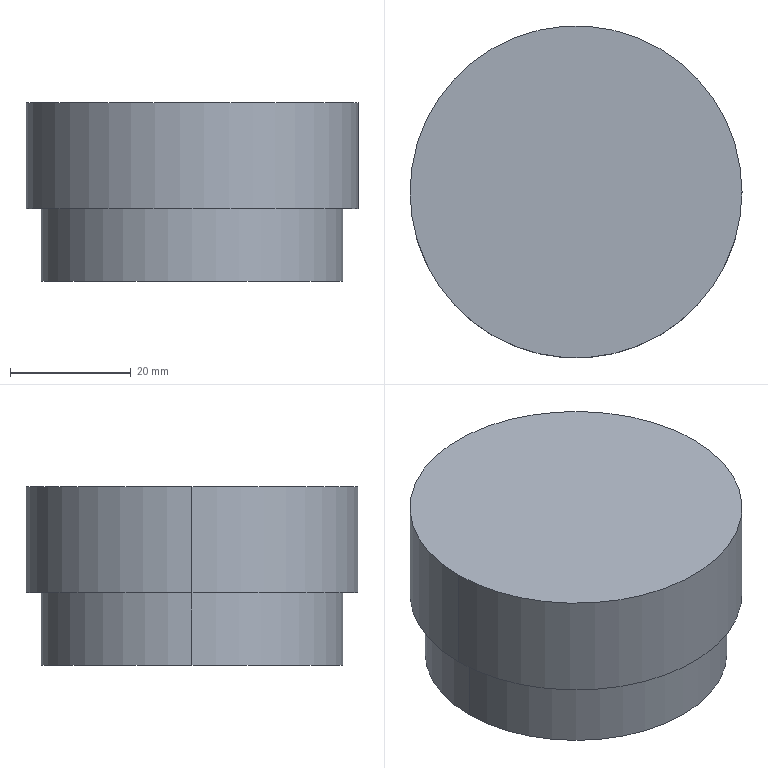Part | SolidWorks | features Extrusion 1, ICE 1 | 1 solid | 7 faces | box 55 x 55 x 29.6 mm | volume 65377 mm3 | cylinder 4 | plane 3 | commonest cylinder face diameters 50 x2 55 x2
STEP:
#1=CARTESIAN_POINT('',(27.5,0.,29.6));
#2=VERTEX_POINT('',#1);
#3=CARTESIAN_POINT('',(-27.5,0.,29.6));
#4=VERTEX_POINT('',#3);
#5=CARTESIAN_POINT('',(0.,0.,29.6));
#6=DIRECTION('',(0.,0.,1.));
#7=DIRECTION('',(1.,0.,0.));
#8=AXIS2_PLACEMENT_3D('',#5,#6,#7);
#9=CIRCLE('',#8,27.5);
#10=EDGE_CURVE('',#2,#4,#9,.T.);
#11=ORIENTED_EDGE('',*,*,#10,.F.);
#12=CARTESIAN_POINT('',(27.5,0.,12.));
#13=VERTEX_POINT('',#12);
#14=CARTESIAN_POINT('',(27.5,0.,29.6));
#15=DIRECTION('',(0.,0.,-1.));
#16=VECTOR('',#15,1000.);
#17=LINE('',#14,#16);
#18=EDGE_CURVE('',#2,#13,#17,.T.);
#19=ORIENTED_EDGE('',*,*,#18,.T.);
#20=CARTESIAN_POINT('',(-27.5,0.,12.));
#21=VERTEX_POINT('',#20);
#22=CARTESIAN_POINT('',(0.,0.,12.));
#23=DIRECTION('',(0.,0.,1.));
#24=DIRECTION('',(1.,0.,0.));
#25=AXIS2_PLACEMENT_3D('',#22,#23,#24);
#26=CIRCLE('',#25,27.5);
#27=EDGE_CURVE('',#13,#21,#26,.T.);
#28=ORIENTED_EDGE('',*,*,#27,.T.);
#29=CARTESIAN_POINT('',(-27.5,0.,29.6));
#30=DIRECTION('',(0.,0.,-1.));
#31=VECTOR('',#30,1000.);
#32=LINE('',#29,#31);
#33=EDGE_CURVE('',#4,#21,#32,.T.);
#34=ORIENTED_EDGE('',*,*,#33,.F.);
#35=EDGE_LOOP('',(#11,#19,#28,#34));
#36=FACE_OUTER_BOUND('',#35,.T.);
#37=CARTESIAN_POINT('',(0.,0.,29.6));
#38=DIRECTION('',(0.,0.,-1.));
#39=DIRECTION('',(-1.,0.,0.));
#40=AXIS2_PLACEMENT_3D('',#37,#38,#39);
#41=CYLINDRICAL_SURFACE('',#40,27.5);
#42=ADVANCED_FACE('',(#36),#41,.T.);
#43=CARTESIAN_POINT('',(25.,0.,12.));
#44=VERTEX_POINT('',#43);
#45=CARTESIAN_POINT('',(-25.,0.,12.));
#46=VERTEX_POINT('',#45);
#47=CARTESIAN_POINT('',(0.,0.,12.));
#48=DIRECTION('',(0.,0.,1.));
#49=DIRECTION('',(1.,0.,0.));
#50=AXIS2_PLACEMENT_3D('',#47,#48,#49);
#51=CIRCLE('',#50,25.);
#52=EDGE_CURVE('',#44,#46,#51,.T.);
#53=ORIENTED_EDGE('',*,*,#52,.F.);
#54=CARTESIAN_POINT('',(25.,0.,0.));
#55=VERTEX_POINT('',#54);
#56=CARTESIAN_POINT('',(25.,0.,12.));
#57=DIRECTION('',(0.,0.,-1.));
#58=VECTOR('',#57,1000.);
#59=LINE('',#56,#58);
#60=EDGE_CURVE('',#44,#55,#59,.T.);
#61=ORIENTED_EDGE('',*,*,#60,.T.);
#62=CARTESIAN_POINT('',(-25.,0.,0.));
#63=VERTEX_POINT('',#62);
#64=CARTESIAN_POINT('',(0.,0.,0.));
#65=DIRECTION('',(0.,0.,1.));
#66=DIRECTION('',(1.,0.,0.));
#67=AXIS2_PLACEMENT_3D('',#64,#65,#66);
#68=CIRCLE('',#67,25.);
#69=EDGE_CURVE('',#55,#63,#68,.T.);
#70=ORIENTED_EDGE('',*,*,#69,.T.);
#71=CARTESIAN_POINT('',(-25.,0.,12.));
#72=DIRECTION('',(0.,0.,-1.));
#73=VECTOR('',#72,1000.);
#74=LINE('',#71,#73);
#75=EDGE_CURVE('',#46,#63,#74,.T.);
#76=ORIENTED_EDGE('',*,*,#75,.F.);
#77=EDGE_LOOP('',(#53,#61,#70,#76));
#78=FACE_OUTER_BOUND('',#77,.T.);
#79=CARTESIAN_POINT('',(0.,0.,12.));
#80=DIRECTION('',(0.,0.,-1.));
#81=DIRECTION('',(-1.,0.,0.));
#82=AXIS2_PLACEMENT_3D('',#79,#80,#81);
#83=CYLINDRICAL_SURFACE('',#82,25.);
#84=ADVANCED_FACE('',(#78),#83,.T.);
#85=ORIENTED_EDGE('',*,*,#60,.F.);
#86=CARTESIAN_POINT('',(0.,0.,12.));
#87=DIRECTION('',(0.,0.,1.));
#88=DIRECTION('',(1.,0.,0.));
#89=AXIS2_PLACEMENT_3D('',#86,#87,#88);
#90=CIRCLE('',#89,25.);
#91=EDGE_CURVE('',#46,#44,#90,.T.);
#92=ORIENTED_EDGE('',*,*,#91,.F.);
#93=ORIENTED_EDGE('',*,*,#75,.T.);
#94=CARTESIAN_POINT('',(0.,0.,0.));
#95=DIRECTION('',(0.,0.,1.));
#96=DIRECTION('',(1.,0.,0.));
#97=AXIS2_PLACEMENT_3D('',#94,#95,#96);
#98=CIRCLE('',#97,25.);
#99=EDGE_CURVE('',#63,#55,#98,.T.);
#100=ORIENTED_EDGE('',*,*,#99,.T.);
#101=EDGE_LOOP('',(#85,#92,#93,#100));
#102=FACE_OUTER_BOUND('',#101,.T.);
#103=CARTESIAN_POINT('',(0.,0.,12.));
#104=DIRECTION('',(0.,0.,-1.));
#105=DIRECTION('',(-1.,0.,0.));
#106=AXIS2_PLACEMENT_3D('',#103,#104,#105);
#107=CYLINDRICAL_SURFACE('',#106,25.);
#108=ADVANCED_FACE('',(#102),#107,.T.);
#109=ORIENTED_EDGE('',*,*,#99,.F.);
#110=ORIENTED_EDGE('',*,*,#69,.F.);
#111=EDGE_LOOP('',(#109,#110));
#112=FACE_OUTER_BOUND('',#111,.T.);
#113=CARTESIAN_POINT('',(0.,0.,0.));
#114=DIRECTION('',(0.,0.,1.));
#115=DIRECTION('',(1.,0.,0.));
#116=AXIS2_PLACEMENT_3D('',#113,#114,#115);
#117=PLANE('',#116);
#118=ADVANCED_FACE('',(#112),#117,.F.);
#119=CARTESIAN_POINT('',(0.,0.,12.));
#120=DIRECTION('',(0.,0.,1.));
#121=DIRECTION('',(1.,0.,0.));
#122=AXIS2_PLACEMENT_3D('',#119,#120,#121);
#123=CIRCLE('',#122,27.5);
#124=EDGE_CURVE('',#21,#13,#123,.T.);
#125=ORIENTED_EDGE('',*,*,#124,.F.);
#126=ORIENTED_EDGE('',*,*,#27,.F.);
#127=EDGE_LOOP('',(#125,#126));
#128=FACE_OUTER_BOUND('',#127,.T.);
#129=ORIENTED_EDGE('',*,*,#91,.T.);
#130=ORIENTED_EDGE('',*,*,#52,.T.);
#131=EDGE_LOOP('',(#129,#130));
#132=FACE_BOUND('',#131,.T.);
#133=CARTESIAN_POINT('',(0.,0.,12.));
#134=DIRECTION('',(0.,0.,1.));
#135=DIRECTION('',(1.,0.,0.));
#136=AXIS2_PLACEMENT_3D('',#133,#134,#135);
#137=PLANE('',#136);
#138=ADVANCED_FACE('',(#128,#132),#137,.F.);
#139=ORIENTED_EDGE('',*,*,#18,.F.);
#140=CARTESIAN_POINT('',(0.,0.,29.6));
#141=DIRECTION('',(0.,0.,1.));
#142=DIRECTION('',(1.,0.,0.));
#143=AXIS2_PLACEMENT_3D('',#140,#141,#142);
#144=CIRCLE('',#143,27.5);
#145=EDGE_CURVE('',#4,#2,#144,.T.);
#146=ORIENTED_EDGE('',*,*,#145,.F.);
#147=ORIENTED_EDGE('',*,*,#33,.T.);
#148=ORIENTED_EDGE('',*,*,#124,.T.);
#149=EDGE_LOOP('',(#139,#146,#147,#148));
#150=FACE_OUTER_BOUND('',#149,.T.);
#151=CARTESIAN_POINT('',(0.,0.,29.6));
#152=DIRECTION('',(0.,0.,-1.));
#153=DIRECTION('',(-1.,0.,0.));
#154=AXIS2_PLACEMENT_3D('',#151,#152,#153);
#155=CYLINDRICAL_SURFACE('',#154,27.5);
#156=ADVANCED_FACE('',(#150),#155,.T.);
#157=ORIENTED_EDGE('',*,*,#145,.T.);
#158=ORIENTED_EDGE('',*,*,#10,.T.);
#159=EDGE_LOOP('',(#157,#158));
#160=FACE_OUTER_BOUND('',#159,.T.);
#161=CARTESIAN_POINT('',(0.,0.,29.6));
#162=DIRECTION('',(0.,0.,1.));
#163=DIRECTION('',(1.,0.,0.));
#164=AXIS2_PLACEMENT_3D('',#161,#162,#163);
#165=PLANE('',#164);
#166=ADVANCED_FACE('',(#160),#165,.T.);
#167=CLOSED_SHELL('',(#42,#84,#108,#118,#138,#156,#166));
#168=MANIFOLD_SOLID_BREP('',#167);
#169=CARTESIAN_POINT('',(0.,0.,0.));
#170=DIRECTION('',(0.,0.,1.));
#171=DIRECTION('',(1.,0.,0.));
#172=AXIS2_PLACEMENT_3D('',#169,#170,#171);
#173=(LENGTH_UNIT()NAMED_UNIT(*)SI_UNIT(.MILLI.,.METRE.));
#174=UNCERTAINTY_MEASURE_WITH_UNIT(LENGTH_MEASURE(0.00001),#173,'','');
#175=(NAMED_UNIT(*)PLANE_ANGLE_UNIT()SI_UNIT($,.RADIAN.));
#176=(NAMED_UNIT(*)SI_UNIT($,.STERADIAN.)SOLID_ANGLE_UNIT());
#177=(GEOMETRIC_REPRESENTATION_CONTEXT(3)GLOBAL_UNCERTAINTY_ASSIGNED_CONTEXT((#174))GLOBAL_UNIT_ASSIGNED_CONTEXT((#173,#175,#176))REPRESENTATION_CONTEXT('',''));
#178=ADVANCED_BREP_SHAPE_REPRESENTATION('',(#168,#172),#177);